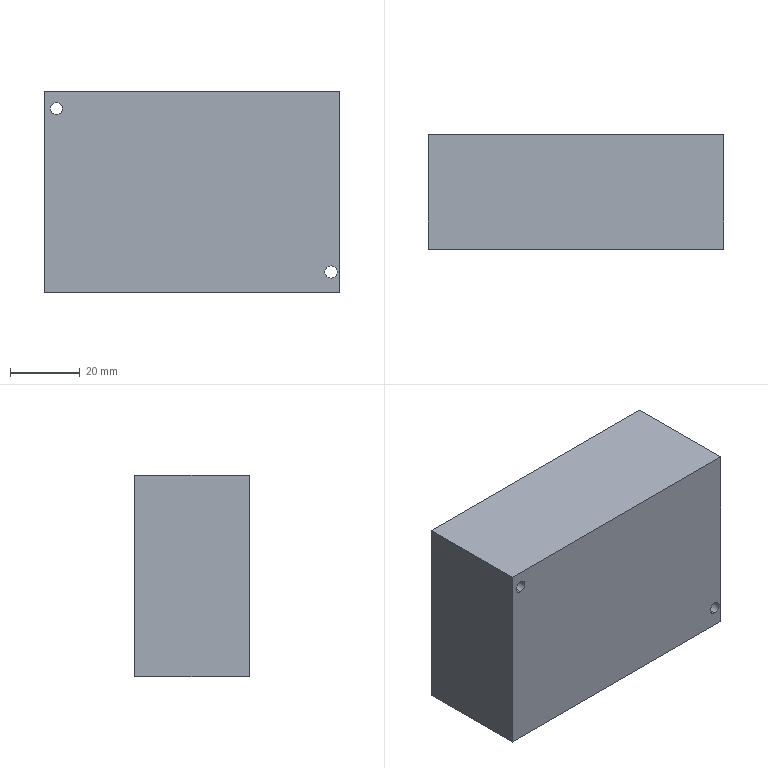Part | 1 solid | 11 faces | box 85 x 33 x 58 mm | volume 162055 mm3 | plane 7 | cylinder 4 | commonest cylinder face diameters 3.5 x4
STEP:
#1=CARTESIAN_POINT('',(-39.,33.,25.75));
#2=VERTEX_POINT('',#1);
#3=CARTESIAN_POINT('',(-40.743,33.,23.845));
#4=VERTEX_POINT('',#3);
#5=CARTESIAN_POINT('',(-39.,33.,24.));
#6=DIRECTION('',(0.,-1.,0.));
#7=DIRECTION('',(0.,0.,-1.));
#8=AXIS2_PLACEMENT_3D('',#5,#6,#7);
#9=CIRCLE('',#8,1.75);
#10=EDGE_CURVE('',#2,#4,#9,.T.);
#11=ORIENTED_EDGE('',*,*,#10,.F.);
#12=CARTESIAN_POINT('',(-39.,0.,25.75));
#13=VERTEX_POINT('',#12);
#14=CARTESIAN_POINT('',(-39.,0.,25.75));
#15=DIRECTION('',(0.,-1.,0.));
#16=VECTOR('',#15,1000.);
#17=LINE('',#14,#16);
#18=EDGE_CURVE('',#2,#13,#17,.T.);
#19=ORIENTED_EDGE('',*,*,#18,.T.);
#20=CARTESIAN_POINT('',(-39.,0.,22.25));
#21=VERTEX_POINT('',#20);
#22=CARTESIAN_POINT('',(-39.,0.,24.));
#23=DIRECTION('',(0.,-1.,0.));
#24=DIRECTION('',(0.,0.,-1.));
#25=AXIS2_PLACEMENT_3D('',#22,#23,#24);
#26=CIRCLE('',#25,1.75);
#27=EDGE_CURVE('',#13,#21,#26,.T.);
#28=ORIENTED_EDGE('',*,*,#27,.T.);
#29=CARTESIAN_POINT('',(-39.,33.,22.25));
#30=VERTEX_POINT('',#29);
#31=CARTESIAN_POINT('',(-39.,0.,22.25));
#32=DIRECTION('',(0.,-1.,0.));
#33=VECTOR('',#32,1000.);
#34=LINE('',#31,#33);
#35=EDGE_CURVE('',#30,#21,#34,.T.);
#36=ORIENTED_EDGE('',*,*,#35,.F.);
#37=CARTESIAN_POINT('',(-39.,33.,24.));
#38=DIRECTION('',(0.,-1.,0.));
#39=DIRECTION('',(0.,0.,-1.));
#40=AXIS2_PLACEMENT_3D('',#37,#38,#39);
#41=CIRCLE('',#40,1.75);
#42=EDGE_CURVE('',#4,#30,#41,.T.);
#43=ORIENTED_EDGE('',*,*,#42,.F.);
#44=EDGE_LOOP('',(#11,#19,#28,#36,#43));
#45=FACE_OUTER_BOUND('',#44,.T.);
#46=CARTESIAN_POINT('',(-39.,0.,24.));
#47=DIRECTION('',(0.,-1.,0.));
#48=DIRECTION('',(0.,0.,-1.));
#49=AXIS2_PLACEMENT_3D('',#46,#47,#48);
#50=CYLINDRICAL_SURFACE('',#49,1.75);
#51=ADVANCED_FACE('',(#45),#50,.F.);
#52=CARTESIAN_POINT('',(40.,33.,-21.25));
#53=VERTEX_POINT('',#52);
#54=CARTESIAN_POINT('',(40.,33.,-24.75));
#55=VERTEX_POINT('',#54);
#56=CARTESIAN_POINT('',(40.,33.,-23.));
#57=DIRECTION('',(0.,-1.,0.));
#58=DIRECTION('',(0.,0.,-1.));
#59=AXIS2_PLACEMENT_3D('',#56,#57,#58);
#60=CIRCLE('',#59,1.75);
#61=EDGE_CURVE('',#53,#55,#60,.T.);
#62=ORIENTED_EDGE('',*,*,#61,.F.);
#63=CARTESIAN_POINT('',(40.,0.,-21.25));
#64=VERTEX_POINT('',#63);
#65=CARTESIAN_POINT('',(40.,0.,-21.25));
#66=DIRECTION('',(0.,-1.,0.));
#67=VECTOR('',#66,1000.);
#68=LINE('',#65,#67);
#69=EDGE_CURVE('',#53,#64,#68,.T.);
#70=ORIENTED_EDGE('',*,*,#69,.T.);
#71=CARTESIAN_POINT('',(40.,0.,-24.75));
#72=VERTEX_POINT('',#71);
#73=CARTESIAN_POINT('',(40.,0.,-23.));
#74=DIRECTION('',(0.,-1.,0.));
#75=DIRECTION('',(0.,0.,-1.));
#76=AXIS2_PLACEMENT_3D('',#73,#74,#75);
#77=CIRCLE('',#76,1.75);
#78=EDGE_CURVE('',#64,#72,#77,.T.);
#79=ORIENTED_EDGE('',*,*,#78,.T.);
#80=CARTESIAN_POINT('',(40.,0.,-24.75));
#81=DIRECTION('',(0.,-1.,0.));
#82=VECTOR('',#81,1000.);
#83=LINE('',#80,#82);
#84=EDGE_CURVE('',#55,#72,#83,.T.);
#85=ORIENTED_EDGE('',*,*,#84,.F.);
#86=EDGE_LOOP('',(#62,#70,#79,#85));
#87=FACE_OUTER_BOUND('',#86,.T.);
#88=CARTESIAN_POINT('',(40.,0.,-23.));
#89=DIRECTION('',(0.,-1.,0.));
#90=DIRECTION('',(0.,0.,-1.));
#91=AXIS2_PLACEMENT_3D('',#88,#89,#90);
#92=CYLINDRICAL_SURFACE('',#91,1.75);
#93=ADVANCED_FACE('',(#87),#92,.F.);
#94=CARTESIAN_POINT('',(-37.257,33.,23.845));
#95=VERTEX_POINT('',#94);
#96=CARTESIAN_POINT('',(-39.,33.,24.));
#97=DIRECTION('',(0.,-1.,0.));
#98=DIRECTION('',(0.,0.,-1.));
#99=AXIS2_PLACEMENT_3D('',#96,#97,#98);
#100=CIRCLE('',#99,1.75);
#101=EDGE_CURVE('',#95,#2,#100,.T.);
#102=ORIENTED_EDGE('',*,*,#101,.T.);
#103=ORIENTED_EDGE('',*,*,#10,.T.);
#104=CARTESIAN_POINT('',(-42.5,33.,23.845));
#105=VERTEX_POINT('',#104);
#106=CARTESIAN_POINT('',(0.,33.,23.845));
#107=DIRECTION('',(-1.,0.,0.));
#108=VECTOR('',#107,1000.);
#109=LINE('',#106,#108);
#110=EDGE_CURVE('',#4,#105,#109,.T.);
#111=ORIENTED_EDGE('',*,*,#110,.T.);
#112=CARTESIAN_POINT('',(-42.5,33.,29.));
#113=VERTEX_POINT('',#112);
#114=CARTESIAN_POINT('',(-42.5,33.,-29.));
#115=DIRECTION('',(0.,0.,1.));
#116=VECTOR('',#115,1000.);
#117=LINE('',#114,#116);
#118=EDGE_CURVE('',#105,#113,#117,.T.);
#119=ORIENTED_EDGE('',*,*,#118,.T.);
#120=CARTESIAN_POINT('',(42.5,33.,29.));
#121=VERTEX_POINT('',#120);
#122=CARTESIAN_POINT('',(-42.5,33.,29.));
#123=DIRECTION('',(1.,0.,0.));
#124=VECTOR('',#123,1000.);
#125=LINE('',#122,#124);
#126=EDGE_CURVE('',#113,#121,#125,.T.);
#127=ORIENTED_EDGE('',*,*,#126,.T.);
#128=CARTESIAN_POINT('',(42.5,33.,-29.));
#129=VERTEX_POINT('',#128);
#130=CARTESIAN_POINT('',(42.5,33.,-29.));
#131=DIRECTION('',(0.,0.,-1.));
#132=VECTOR('',#131,1000.);
#133=LINE('',#130,#132);
#134=EDGE_CURVE('',#121,#129,#133,.T.);
#135=ORIENTED_EDGE('',*,*,#134,.T.);
#136=CARTESIAN_POINT('',(-25.098,33.,-29.));
#137=VERTEX_POINT('',#136);
#138=CARTESIAN_POINT('',(-42.5,33.,-29.));
#139=DIRECTION('',(-1.,0.,0.));
#140=VECTOR('',#139,1000.);
#141=LINE('',#138,#140);
#142=EDGE_CURVE('',#129,#137,#141,.T.);
#143=ORIENTED_EDGE('',*,*,#142,.T.);
#144=CARTESIAN_POINT('',(-25.098,33.,23.845));
#145=VERTEX_POINT('',#144);
#146=CARTESIAN_POINT('',(-25.098,33.,0.));
#147=DIRECTION('',(0.,0.,1.));
#148=VECTOR('',#147,1000.);
#149=LINE('',#146,#148);
#150=EDGE_CURVE('',#137,#145,#149,.T.);
#151=ORIENTED_EDGE('',*,*,#150,.T.);
#152=CARTESIAN_POINT('',(0.,33.,23.845));
#153=DIRECTION('',(-1.,0.,0.));
#154=VECTOR('',#153,1000.);
#155=LINE('',#152,#154);
#156=EDGE_CURVE('',#145,#95,#155,.T.);
#157=ORIENTED_EDGE('',*,*,#156,.T.);
#158=EDGE_LOOP('',(#102,#103,#111,#119,#127,#135,#143,#151,#157));
#159=FACE_OUTER_BOUND('',#158,.T.);
#160=CARTESIAN_POINT('',(40.,33.,-23.));
#161=DIRECTION('',(0.,-1.,0.));
#162=DIRECTION('',(0.,0.,-1.));
#163=AXIS2_PLACEMENT_3D('',#160,#161,#162);
#164=CIRCLE('',#163,1.75);
#165=EDGE_CURVE('',#55,#53,#164,.T.);
#166=ORIENTED_EDGE('',*,*,#165,.T.);
#167=ORIENTED_EDGE('',*,*,#61,.T.);
#168=EDGE_LOOP('',(#166,#167));
#169=FACE_BOUND('',#168,.T.);
#170=CARTESIAN_POINT('',(0.,33.,0.));
#171=DIRECTION('',(0.,1.,0.));
#172=DIRECTION('',(0.,0.,1.));
#173=AXIS2_PLACEMENT_3D('',#170,#171,#172);
#174=PLANE('',#173);
#175=ADVANCED_FACE('',(#159,#169),#174,.T.);
#176=CARTESIAN_POINT('',(42.5,0.,29.));
#177=VERTEX_POINT('',#176);
#178=CARTESIAN_POINT('',(42.5,0.,-29.));
#179=VERTEX_POINT('',#178);
#180=CARTESIAN_POINT('',(42.5,0.,-29.));
#181=DIRECTION('',(0.,0.,-1.));
#182=VECTOR('',#181,1000.);
#183=LINE('',#180,#182);
#184=EDGE_CURVE('',#177,#179,#183,.T.);
#185=ORIENTED_EDGE('',*,*,#184,.T.);
#186=CARTESIAN_POINT('',(42.5,33.,-29.));
#187=DIRECTION('',(0.,-1.,0.));
#188=VECTOR('',#187,1000.);
#189=LINE('',#186,#188);
#190=EDGE_CURVE('',#129,#179,#189,.T.);
#191=ORIENTED_EDGE('',*,*,#190,.F.);
#192=ORIENTED_EDGE('',*,*,#134,.F.);
#193=CARTESIAN_POINT('',(42.5,33.,29.));
#194=DIRECTION('',(0.,-1.,0.));
#195=VECTOR('',#194,1000.);
#196=LINE('',#193,#195);
#197=EDGE_CURVE('',#121,#177,#196,.T.);
#198=ORIENTED_EDGE('',*,*,#197,.T.);
#199=EDGE_LOOP('',(#185,#191,#192,#198));
#200=FACE_OUTER_BOUND('',#199,.T.);
#201=CARTESIAN_POINT('',(42.5,33.,-29.));
#202=DIRECTION('',(-1.,0.,0.));
#203=DIRECTION('',(0.,0.,1.));
#204=AXIS2_PLACEMENT_3D('',#201,#202,#203);
#205=PLANE('',#204);
#206=ADVANCED_FACE('',(#200),#205,.F.);
#207=CARTESIAN_POINT('',(-42.5,0.,-29.));
#208=VERTEX_POINT('',#207);
#209=CARTESIAN_POINT('',(-42.5,0.,-29.));
#210=DIRECTION('',(-1.,0.,0.));
#211=VECTOR('',#210,1000.);
#212=LINE('',#209,#211);
#213=EDGE_CURVE('',#179,#208,#212,.T.);
#214=ORIENTED_EDGE('',*,*,#213,.T.);
#215=CARTESIAN_POINT('',(-42.5,33.,-29.));
#216=VERTEX_POINT('',#215);
#217=CARTESIAN_POINT('',(-42.5,33.,-29.));
#218=DIRECTION('',(0.,-1.,0.));
#219=VECTOR('',#218,1000.);
#220=LINE('',#217,#219);
#221=EDGE_CURVE('',#216,#208,#220,.T.);
#222=ORIENTED_EDGE('',*,*,#221,.F.);
#223=CARTESIAN_POINT('',(-42.5,33.,-29.));
#224=DIRECTION('',(-1.,0.,0.));
#225=VECTOR('',#224,1000.);
#226=LINE('',#223,#225);
#227=EDGE_CURVE('',#137,#216,#226,.T.);
#228=ORIENTED_EDGE('',*,*,#227,.F.);
#229=ORIENTED_EDGE('',*,*,#142,.F.);
#230=ORIENTED_EDGE('',*,*,#190,.T.);
#231=EDGE_LOOP('',(#214,#222,#228,#229,#230));
#232=FACE_OUTER_BOUND('',#231,.T.);
#233=CARTESIAN_POINT('',(-42.5,33.,-29.));
#234=DIRECTION('',(0.,0.,1.));
#235=DIRECTION('',(1.,0.,0.));
#236=AXIS2_PLACEMENT_3D('',#233,#234,#235);
#237=PLANE('',#236);
#238=ADVANCED_FACE('',(#232),#237,.F.);
#239=CARTESIAN_POINT('',(-42.5,0.,29.));
#240=VERTEX_POINT('',#239);
#241=CARTESIAN_POINT('',(-42.5,0.,-29.));
#242=DIRECTION('',(0.,0.,1.));
#243=VECTOR('',#242,1000.);
#244=LINE('',#241,#243);
#245=EDGE_CURVE('',#208,#240,#244,.T.);
#246=ORIENTED_EDGE('',*,*,#245,.T.);
#247=CARTESIAN_POINT('',(-42.5,33.,29.));
#248=DIRECTION('',(0.,-1.,0.));
#249=VECTOR('',#248,1000.);
#250=LINE('',#247,#249);
#251=EDGE_CURVE('',#113,#240,#250,.T.);
#252=ORIENTED_EDGE('',*,*,#251,.F.);
#253=ORIENTED_EDGE('',*,*,#118,.F.);
#254=CARTESIAN_POINT('',(-42.5,33.,-29.));
#255=DIRECTION('',(0.,0.,1.));
#256=VECTOR('',#255,1000.);
#257=LINE('',#254,#256);
#258=EDGE_CURVE('',#216,#105,#257,.T.);
#259=ORIENTED_EDGE('',*,*,#258,.F.);
#260=ORIENTED_EDGE('',*,*,#221,.T.);
#261=EDGE_LOOP('',(#246,#252,#253,#259,#260));
#262=FACE_OUTER_BOUND('',#261,.T.);
#263=CARTESIAN_POINT('',(-42.5,33.,-29.));
#264=DIRECTION('',(1.,0.,0.));
#265=DIRECTION('',(0.,0.,-1.));
#266=AXIS2_PLACEMENT_3D('',#263,#264,#265);
#267=PLANE('',#266);
#268=ADVANCED_FACE('',(#262),#267,.F.);
#269=CARTESIAN_POINT('',(-42.5,0.,29.));
#270=DIRECTION('',(1.,0.,0.));
#271=VECTOR('',#270,1000.);
#272=LINE('',#269,#271);
#273=EDGE_CURVE('',#240,#177,#272,.T.);
#274=ORIENTED_EDGE('',*,*,#273,.T.);
#275=ORIENTED_EDGE('',*,*,#197,.F.);
#276=ORIENTED_EDGE('',*,*,#126,.F.);
#277=ORIENTED_EDGE('',*,*,#251,.T.);
#278=EDGE_LOOP('',(#274,#275,#276,#277));
#279=FACE_OUTER_BOUND('',#278,.T.);
#280=CARTESIAN_POINT('',(-42.5,33.,29.));
#281=DIRECTION('',(0.,0.,-1.));
#282=DIRECTION('',(-1.,0.,0.));
#283=AXIS2_PLACEMENT_3D('',#280,#281,#282);
#284=PLANE('',#283);
#285=ADVANCED_FACE('',(#279),#284,.F.);
#286=ORIENTED_EDGE('',*,*,#42,.T.);
#287=CARTESIAN_POINT('',(-39.,33.,24.));
#288=DIRECTION('',(0.,-1.,0.));
#289=DIRECTION('',(0.,0.,-1.));
#290=AXIS2_PLACEMENT_3D('',#287,#288,#289);
#291=CIRCLE('',#290,1.75);
#292=EDGE_CURVE('',#30,#95,#291,.T.);
#293=ORIENTED_EDGE('',*,*,#292,.T.);
#294=ORIENTED_EDGE('',*,*,#156,.F.);
#295=ORIENTED_EDGE('',*,*,#150,.F.);
#296=ORIENTED_EDGE('',*,*,#227,.T.);
#297=ORIENTED_EDGE('',*,*,#258,.T.);
#298=ORIENTED_EDGE('',*,*,#110,.F.);
#299=EDGE_LOOP('',(#286,#293,#294,#295,#296,#297,#298));
#300=FACE_OUTER_BOUND('',#299,.T.);
#301=CARTESIAN_POINT('',(0.,33.,0.));
#302=DIRECTION('',(0.,1.,0.));
#303=DIRECTION('',(0.,0.,1.));
#304=AXIS2_PLACEMENT_3D('',#301,#302,#303);
#305=PLANE('',#304);
#306=ADVANCED_FACE('',(#300),#305,.T.);
#307=CARTESIAN_POINT('',(-39.,0.,24.));
#308=DIRECTION('',(0.,-1.,0.));
#309=DIRECTION('',(0.,0.,-1.));
#310=AXIS2_PLACEMENT_3D('',#307,#308,#309);
#311=CIRCLE('',#310,1.75);
#312=EDGE_CURVE('',#21,#13,#311,.T.);
#313=ORIENTED_EDGE('',*,*,#312,.F.);
#314=ORIENTED_EDGE('',*,*,#27,.F.);
#315=EDGE_LOOP('',(#313,#314));
#316=FACE_BOUND('',#315,.T.);
#317=CARTESIAN_POINT('',(40.,0.,-23.));
#318=DIRECTION('',(0.,-1.,0.));
#319=DIRECTION('',(0.,0.,-1.));
#320=AXIS2_PLACEMENT_3D('',#317,#318,#319);
#321=CIRCLE('',#320,1.75);
#322=EDGE_CURVE('',#72,#64,#321,.T.);
#323=ORIENTED_EDGE('',*,*,#322,.F.);
#324=ORIENTED_EDGE('',*,*,#78,.F.);
#325=EDGE_LOOP('',(#323,#324));
#326=FACE_BOUND('',#325,.T.);
#327=ORIENTED_EDGE('',*,*,#184,.F.);
#328=ORIENTED_EDGE('',*,*,#273,.F.);
#329=ORIENTED_EDGE('',*,*,#245,.F.);
#330=ORIENTED_EDGE('',*,*,#213,.F.);
#331=EDGE_LOOP('',(#327,#328,#329,#330));
#332=FACE_OUTER_BOUND('',#331,.T.);
#333=CARTESIAN_POINT('',(0.,0.,0.));
#334=DIRECTION('',(0.,1.,0.));
#335=DIRECTION('',(0.,0.,1.));
#336=AXIS2_PLACEMENT_3D('',#333,#334,#335);
#337=PLANE('',#336);
#338=ADVANCED_FACE('',(#316,#326,#332),#337,.F.);
#339=ORIENTED_EDGE('',*,*,#69,.F.);
#340=ORIENTED_EDGE('',*,*,#165,.F.);
#341=ORIENTED_EDGE('',*,*,#84,.T.);
#342=ORIENTED_EDGE('',*,*,#322,.T.);
#343=EDGE_LOOP('',(#339,#340,#341,#342));
#344=FACE_OUTER_BOUND('',#343,.T.);
#345=CARTESIAN_POINT('',(40.,0.,-23.));
#346=DIRECTION('',(0.,-1.,0.));
#347=DIRECTION('',(0.,0.,-1.));
#348=AXIS2_PLACEMENT_3D('',#345,#346,#347);
#349=CYLINDRICAL_SURFACE('',#348,1.75);
#350=ADVANCED_FACE('',(#344),#349,.F.);
#351=ORIENTED_EDGE('',*,*,#18,.F.);
#352=ORIENTED_EDGE('',*,*,#101,.F.);
#353=ORIENTED_EDGE('',*,*,#292,.F.);
#354=ORIENTED_EDGE('',*,*,#35,.T.);
#355=ORIENTED_EDGE('',*,*,#312,.T.);
#356=EDGE_LOOP('',(#351,#352,#353,#354,#355));
#357=FACE_OUTER_BOUND('',#356,.T.);
#358=CARTESIAN_POINT('',(-39.,0.,24.));
#359=DIRECTION('',(0.,-1.,0.));
#360=DIRECTION('',(0.,0.,-1.));
#361=AXIS2_PLACEMENT_3D('',#358,#359,#360);
#362=CYLINDRICAL_SURFACE('',#361,1.75);
#363=ADVANCED_FACE('',(#357),#362,.F.);
#364=CLOSED_SHELL('',(#51,#93,#175,#206,#238,#268,#285,#306,#338,#350,#363));
#365=MANIFOLD_SOLID_BREP('',#364);
#366=CARTESIAN_POINT('',(0.,0.,0.));
#367=DIRECTION('',(0.,0.,1.));
#368=DIRECTION('',(1.,0.,0.));
#369=AXIS2_PLACEMENT_3D('',#366,#367,#368);
#370=(LENGTH_UNIT()NAMED_UNIT(*)SI_UNIT(.MILLI.,.METRE.));
#371=UNCERTAINTY_MEASURE_WITH_UNIT(LENGTH_MEASURE(0.00001),#370,'','');
#372=(NAMED_UNIT(*)PLANE_ANGLE_UNIT()SI_UNIT($,.RADIAN.));
#373=(NAMED_UNIT(*)SI_UNIT($,.STERADIAN.)SOLID_ANGLE_UNIT());
#374=(GEOMETRIC_REPRESENTATION_CONTEXT(3)GLOBAL_UNCERTAINTY_ASSIGNED_CONTEXT((#371))GLOBAL_UNIT_ASSIGNED_CONTEXT((#370,#372,#373))REPRESENTATION_CONTEXT('',''));
#375=ADVANCED_BREP_SHAPE_REPRESENTATION('',(#365,#369),#374);